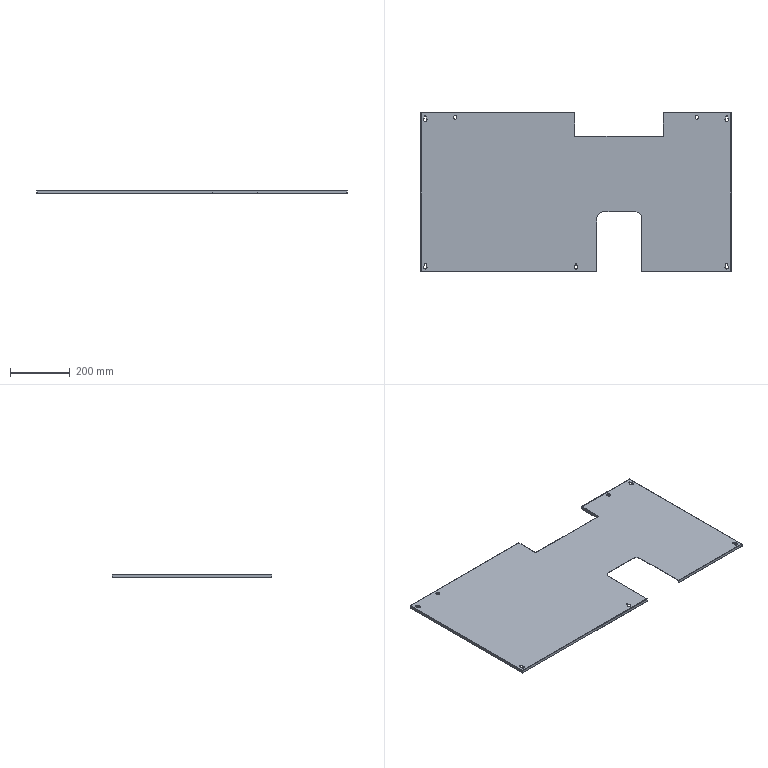Part | NX | features BREP 1 | 1 solid | 75 faces | box 1040 x 534 x 10 mm | volume 790797 mm3 | cylinder 38 | plane 34 | sphere 3 | commonest cylinder face diameters 12 x19 2 x12 6 x5 40 x2